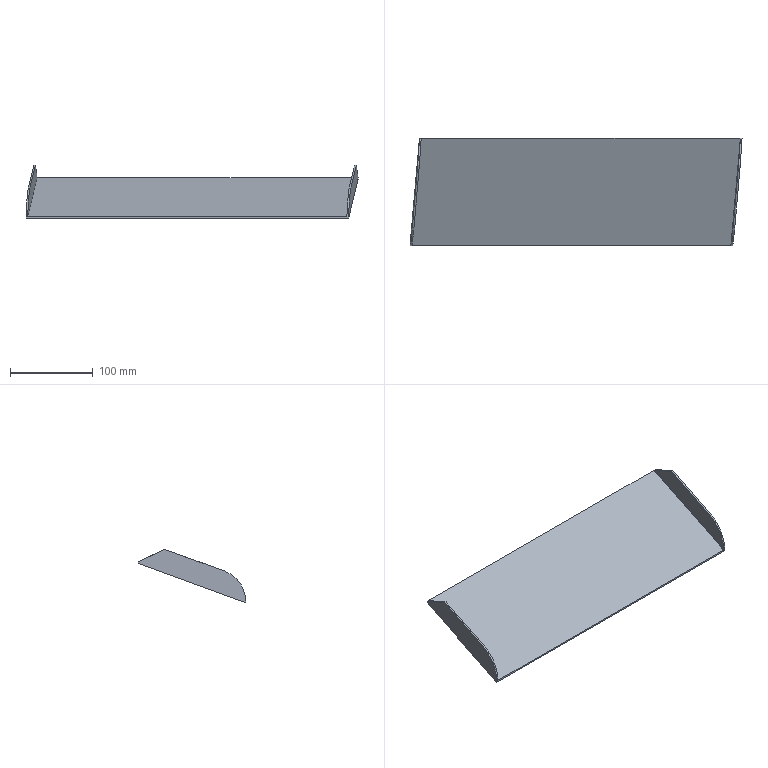Part | NX | features solid 2 | 1 solid | 16 faces | box 400.371 x 130.154 x 64.471 mm | volume 119225 mm3 | plane 14 | cylinder 2 | commonest cylinder face diameters 80 x2
STEP:
#1=CARTESIAN_POINT('',(-476.319,-520.,-137.863));
#2=VERTEX_POINT('',#1);
#3=CARTESIAN_POINT('',(-478.326,-520.,-137.863));
#4=VERTEX_POINT('',#3);
#5=CARTESIAN_POINT('',(-862.915,-520.,-137.863));
#6=DIRECTION('',(1.,0.,0.));
#7=VECTOR('',#6,1000.);
#8=LINE('',#5,#7);
#9=EDGE_CURVE('',#2,#4,#8,.F.);
#10=ORIENTED_EDGE('',*,*,#9,.F.);
#11=CARTESIAN_POINT('',(-476.319,-520.,-139.992));
#12=VERTEX_POINT('',#11);
#13=CARTESIAN_POINT('',(-476.319,-520.,-105.));
#14=DIRECTION('',(0.,0.,1.));
#15=VECTOR('',#14,1000.);
#16=LINE('',#13,#15);
#17=EDGE_CURVE('',#2,#12,#16,.F.);
#18=ORIENTED_EDGE('',*,*,#17,.T.);
#19=CARTESIAN_POINT('',(-865.317,-520.,-139.992));
#20=VERTEX_POINT('',#19);
#21=CARTESIAN_POINT('',(-862.915,-520.,-139.992));
#22=DIRECTION('',(1.,0.,0.));
#23=VECTOR('',#22,1000.);
#24=LINE('',#21,#23);
#25=EDGE_CURVE('',#20,#12,#24,.T.);
#26=ORIENTED_EDGE('',*,*,#25,.F.);
#27=CARTESIAN_POINT('',(-865.257,-520.,-137.863));
#28=VERTEX_POINT('',#27);
#29=CARTESIAN_POINT('',(-865.034,-520.,-129.94));
#30=DIRECTION('',(-0.02811,0.,-0.9996));
#31=VECTOR('',#30,1000.);
#32=LINE('',#29,#31);
#33=EDGE_CURVE('',#28,#20,#32,.T.);
#34=ORIENTED_EDGE('',*,*,#33,.F.);
#35=CARTESIAN_POINT('',(-862.915,-520.,-137.863));
#36=DIRECTION('',(1.,0.,0.));
#37=VECTOR('',#36,1000.);
#38=LINE('',#35,#37);
#39=EDGE_CURVE('',#4,#28,#38,.F.);
#40=ORIENTED_EDGE('',*,*,#39,.F.);
#41=EDGE_LOOP('',(#10,#18,#26,#34,#40));
#42=FACE_BOUND('',#41,.T.);
#43=CARTESIAN_POINT('',(-395.,-520.,0.));
#44=DIRECTION('',(0.,1.,0.));
#45=DIRECTION('',(0.,0.,1.));
#46=AXIS2_PLACEMENT_3D('',#43,#44,#45);
#47=PLANE('',#46);
#48=ADVANCED_FACE('',(#42),#47,.T.);
#49=CARTESIAN_POINT('',(-876.69,-650.,-187.308));
#50=VERTEX_POINT('',#49);
#51=CARTESIAN_POINT('',(-876.63,-650.,-185.179));
#52=VERTEX_POINT('',#51);
#53=CARTESIAN_POINT('',(-875.069,-650.,-129.658));
#54=DIRECTION('',(-0.02811,0.,-0.9996));
#55=VECTOR('',#54,1000.);
#56=LINE('',#53,#55);
#57=EDGE_CURVE('',#50,#52,#56,.F.);
#58=ORIENTED_EDGE('',*,*,#57,.F.);
#59=CARTESIAN_POINT('',(-487.693,-650.,-187.308));
#60=VERTEX_POINT('',#59);
#61=CARTESIAN_POINT('',(50.,-650.,-187.308));
#62=DIRECTION('',(-1.,0.,0.));
#63=VECTOR('',#62,1000.);
#64=LINE('',#61,#63);
#65=EDGE_CURVE('',#50,#60,#64,.F.);
#66=ORIENTED_EDGE('',*,*,#65,.T.);
#67=CARTESIAN_POINT('',(-487.693,-650.,-185.179));
#68=VERTEX_POINT('',#67);
#69=CARTESIAN_POINT('',(-487.693,-650.,-105.));
#70=DIRECTION('',(0.,0.,1.));
#71=VECTOR('',#70,1000.);
#72=LINE('',#69,#71);
#73=EDGE_CURVE('',#60,#68,#72,.T.);
#74=ORIENTED_EDGE('',*,*,#73,.T.);
#75=CARTESIAN_POINT('',(-489.699,-650.,-185.179));
#76=VERTEX_POINT('',#75);
#77=CARTESIAN_POINT('',(-476.319,-650.,-185.179));
#78=DIRECTION('',(1.,0.,0.));
#79=VECTOR('',#78,1000.);
#80=LINE('',#77,#79);
#81=EDGE_CURVE('',#68,#76,#80,.F.);
#82=ORIENTED_EDGE('',*,*,#81,.T.);
#83=CARTESIAN_POINT('',(-874.624,-650.,-185.179));
#84=VERTEX_POINT('',#83);
#85=CARTESIAN_POINT('',(-862.915,-650.,-185.179));
#86=DIRECTION('',(1.,0.,0.));
#87=VECTOR('',#86,1000.);
#88=LINE('',#85,#87);
#89=EDGE_CURVE('',#84,#76,#88,.T.);
#90=ORIENTED_EDGE('',*,*,#89,.F.);
#91=CARTESIAN_POINT('',(-862.915,-650.,-185.179));
#92=DIRECTION('',(1.,0.,0.));
#93=VECTOR('',#92,1000.);
#94=LINE('',#91,#93);
#95=EDGE_CURVE('',#52,#84,#94,.T.);
#96=ORIENTED_EDGE('',*,*,#95,.F.);
#97=EDGE_LOOP('',(#58,#66,#74,#82,#90,#96));
#98=FACE_BOUND('',#97,.T.);
#99=CARTESIAN_POINT('',(50.,-650.,-570.));
#100=DIRECTION('',(0.,1.,0.));
#101=DIRECTION('',(-1.,0.,0.));
#102=AXIS2_PLACEMENT_3D('',#99,#100,#101);
#103=PLANE('',#102);
#104=ADVANCED_FACE('',(#98),#103,.F.);
#105=CARTESIAN_POINT('',(-867.305,-551.964,-122.893));
#106=VERTEX_POINT('',#105);
#107=CARTESIAN_POINT('',(-873.582,-623.706,-149.005));
#108=VERTEX_POINT('',#107);
#109=CARTESIAN_POINT('',(-865.257,-528.551,-114.371));
#110=DIRECTION('',(-0.08194,-0.9365,-0.3409));
#111=VECTOR('',#110,1000.);
#112=LINE('',#109,#111);
#113=EDGE_CURVE('',#106,#108,#112,.T.);
#114=ORIENTED_EDGE('',*,*,#113,.F.);
#115=CARTESIAN_POINT('',(-864.004,-500.45,-147.02));
#116=DIRECTION('',(-0.05794,-0.9041,0.4234));
#117=VECTOR('',#116,1000.);
#118=LINE('',#115,#117);
#119=EDGE_CURVE('',#106,#28,#118,.F.);
#120=ORIENTED_EDGE('',*,*,#119,.T.);
#121=ORIENTED_EDGE('',*,*,#33,.T.);
#122=CARTESIAN_POINT('',(-862.915,-492.548,-130.));
#123=DIRECTION('',(-0.08194,-0.9365,-0.3409));
#124=VECTOR('',#123,1000.);
#125=LINE('',#122,#124);
#126=EDGE_CURVE('',#20,#50,#125,.T.);
#127=ORIENTED_EDGE('',*,*,#126,.T.);
#128=ORIENTED_EDGE('',*,*,#57,.T.);
#129=CARTESIAN_POINT('',(-873.582,-610.025,-186.592));
#130=DIRECTION('',(-0.9966,0.07699,0.02802));
#131=DIRECTION('',(-0.08194,-0.9365,-0.3409));
#132=AXIS2_PLACEMENT_3D('',#129,#130,#131);
#133=ELLIPSE('',#132,40.135,40.);
#134=EDGE_CURVE('',#52,#108,#133,.T.);
#135=ORIENTED_EDGE('',*,*,#134,.T.);
#136=EDGE_LOOP('',(#114,#120,#121,#127,#128,#135));
#137=FACE_BOUND('',#136,.T.);
#138=CARTESIAN_POINT('',(-862.915,-492.548,-130.));
#139=DIRECTION('',(-0.9966,0.07699,0.02802));
#140=DIRECTION('',(-0.07702,-0.997,0.));
#141=AXIS2_PLACEMENT_3D('',#138,#139,#140);
#142=PLANE('',#141);
#143=ADVANCED_FACE('',(#137),#142,.T.);
#144=ORIENTED_EDGE('',*,*,#17,.F.);
#145=CARTESIAN_POINT('',(-476.588,-523.078,-138.983));
#146=DIRECTION('',(-0.08194,-0.9365,-0.3409));
#147=VECTOR('',#146,1000.);
#148=LINE('',#145,#147);
#149=EDGE_CURVE('',#2,#68,#148,.T.);
#150=ORIENTED_EDGE('',*,*,#149,.T.);
#151=ORIENTED_EDGE('',*,*,#73,.F.);
#152=CARTESIAN_POINT('',(-481.762,-582.21,-162.634));
#153=DIRECTION('',(0.08194,0.9365,0.3409));
#154=VECTOR('',#153,1000.);
#155=LINE('',#152,#154);
#156=EDGE_CURVE('',#12,#60,#155,.F.);
#157=ORIENTED_EDGE('',*,*,#156,.F.);
#158=EDGE_LOOP('',(#144,#150,#151,#157));
#159=FACE_BOUND('',#158,.T.);
#160=CARTESIAN_POINT('',(-483.583,-603.028,-105.));
#161=DIRECTION('',(0.9962,-0.08716,0.));
#162=DIRECTION('',(0.08716,0.9962,0.));
#163=AXIS2_PLACEMENT_3D('',#160,#161,#162);
#164=PLANE('',#163);
#165=ADVANCED_FACE('',(#159),#164,.T.);
#166=CARTESIAN_POINT('',(-478.582,-522.924,-138.927));
#167=DIRECTION('',(0.08194,0.9365,0.3409));
#168=VECTOR('',#167,1000.);
#169=LINE('',#166,#168);
#170=EDGE_CURVE('',#4,#76,#169,.F.);
#171=ORIENTED_EDGE('',*,*,#170,.F.);
#172=ORIENTED_EDGE('',*,*,#39,.T.);
#173=CARTESIAN_POINT('',(-863.264,-520.154,-137.919));
#174=VERTEX_POINT('',#173);
#175=CARTESIAN_POINT('',(-865.257,-520.,-137.863));
#176=DIRECTION('',(0.9966,-0.07699,-0.02802));
#177=VECTOR('',#176,1000.);
#178=LINE('',#175,#177);
#179=EDGE_CURVE('',#28,#174,#178,.T.);
#180=ORIENTED_EDGE('',*,*,#179,.T.);
#181=CARTESIAN_POINT('',(-863.264,-520.154,-137.919));
#182=DIRECTION('',(-0.08194,-0.9365,-0.3409));
#183=VECTOR('',#182,1000.);
#184=LINE('',#181,#183);
#185=EDGE_CURVE('',#174,#84,#184,.T.);
#186=ORIENTED_EDGE('',*,*,#185,.T.);
#187=ORIENTED_EDGE('',*,*,#89,.T.);
#188=EDGE_LOOP('',(#171,#172,#180,#186,#187));
#189=FACE_BOUND('',#188,.T.);
#190=CARTESIAN_POINT('',(-862.915,-493.232,-128.121));
#191=DIRECTION('',(0.,0.342,-0.9397));
#192=DIRECTION('',(-0.08194,-0.9365,-0.3409));
#193=AXIS2_PLACEMENT_3D('',#190,#191,#192);
#194=PLANE('',#193);
#195=ADVANCED_FACE('',(#189),#194,.F.);
#196=ORIENTED_EDGE('',*,*,#126,.F.);
#197=ORIENTED_EDGE('',*,*,#25,.T.);
#198=ORIENTED_EDGE('',*,*,#156,.T.);
#199=ORIENTED_EDGE('',*,*,#65,.F.);
#200=EDGE_LOOP('',(#196,#197,#198,#199));
#201=FACE_BOUND('',#200,.T.);
#202=CARTESIAN_POINT('',(-862.915,-492.548,-130.));
#203=DIRECTION('',(0.,0.342,-0.9397));
#204=DIRECTION('',(-0.08194,-0.9365,-0.3409));
#205=AXIS2_PLACEMENT_3D('',#202,#203,#204);
#206=PLANE('',#205);
#207=ADVANCED_FACE('',(#201),#206,.T.);
#208=CARTESIAN_POINT('',(-865.312,-552.118,-122.949));
#209=VERTEX_POINT('',#208);
#210=CARTESIAN_POINT('',(-871.575,-623.706,-149.005));
#211=VERTEX_POINT('',#210);
#212=CARTESIAN_POINT('',(-863.264,-528.704,-114.427));
#213=DIRECTION('',(-0.08194,-0.9365,-0.3409));
#214=VECTOR('',#213,1000.);
#215=LINE('',#212,#214);
#216=EDGE_CURVE('',#209,#211,#215,.T.);
#217=ORIENTED_EDGE('',*,*,#216,.F.);
#218=CARTESIAN_POINT('',(-867.305,-551.964,-122.893));
#219=DIRECTION('',(0.9966,-0.07699,-0.02802));
#220=VECTOR('',#219,1000.);
#221=LINE('',#218,#220);
#222=EDGE_CURVE('',#209,#106,#221,.F.);
#223=ORIENTED_EDGE('',*,*,#222,.T.);
#224=ORIENTED_EDGE('',*,*,#113,.T.);
#225=CARTESIAN_POINT('',(-873.875,-623.706,-149.005));
#226=DIRECTION('',(-1.,0.,0.));
#227=VECTOR('',#226,1000.);
#228=LINE('',#225,#227);
#229=EDGE_CURVE('',#108,#211,#228,.F.);
#230=ORIENTED_EDGE('',*,*,#229,.T.);
#231=EDGE_LOOP('',(#217,#223,#224,#230));
#232=FACE_BOUND('',#231,.T.);
#233=CARTESIAN_POINT('',(-865.257,-528.551,-114.371));
#234=DIRECTION('',(0.,0.342,-0.9397));
#235=DIRECTION('',(-0.08194,-0.9365,-0.3409));
#236=AXIS2_PLACEMENT_3D('',#233,#234,#235);
#237=PLANE('',#236);
#238=ADVANCED_FACE('',(#232),#237,.F.);
#239=ORIENTED_EDGE('',*,*,#185,.F.);
#240=CARTESIAN_POINT('',(-863.264,-520.154,-137.919));
#241=DIRECTION('',(0.05794,0.9041,-0.4234));
#242=VECTOR('',#241,1000.);
#243=LINE('',#240,#242);
#244=EDGE_CURVE('',#174,#209,#243,.F.);
#245=ORIENTED_EDGE('',*,*,#244,.T.);
#246=ORIENTED_EDGE('',*,*,#216,.T.);
#247=CARTESIAN_POINT('',(-871.575,-610.025,-186.592));
#248=DIRECTION('',(-0.9966,0.07699,0.02802));
#249=DIRECTION('',(-0.08194,-0.9365,-0.3409));
#250=AXIS2_PLACEMENT_3D('',#247,#248,#249);
#251=ELLIPSE('',#250,40.135,40.);
#252=EDGE_CURVE('',#211,#84,#251,.F.);
#253=ORIENTED_EDGE('',*,*,#252,.T.);
#254=EDGE_LOOP('',(#239,#245,#246,#253));
#255=FACE_BOUND('',#254,.T.);
#256=CARTESIAN_POINT('',(-863.264,-520.154,-137.919));
#257=DIRECTION('',(-0.9966,0.07699,0.02802));
#258=DIRECTION('',(-0.07702,-0.997,0.));
#259=AXIS2_PLACEMENT_3D('',#256,#257,#258);
#260=PLANE('',#259);
#261=ADVANCED_FACE('',(#255),#260,.F.);
#262=ORIENTED_EDGE('',*,*,#134,.F.);
#263=ORIENTED_EDGE('',*,*,#95,.T.);
#264=ORIENTED_EDGE('',*,*,#252,.F.);
#265=ORIENTED_EDGE('',*,*,#229,.F.);
#266=EDGE_LOOP('',(#262,#263,#264,#265));
#267=FACE_BOUND('',#266,.T.);
#268=CARTESIAN_POINT('',(50.,-610.025,-186.592));
#269=DIRECTION('',(-1.,0.,0.));
#270=DIRECTION('',(0.,0.,1.));
#271=AXIS2_PLACEMENT_3D('',#268,#269,#270);
#272=CYLINDRICAL_SURFACE('',#271,40.);
#273=ADVANCED_FACE('',(#267),#272,.T.);
#274=ORIENTED_EDGE('',*,*,#9,.T.);
#275=CARTESIAN_POINT('',(-478.312,-519.846,-137.807));
#276=VERTEX_POINT('',#275);
#277=CARTESIAN_POINT('',(-478.312,-519.846,-137.807));
#278=DIRECTION('',(-0.08194,-0.9365,-0.3409));
#279=VECTOR('',#278,1000.);
#280=LINE('',#277,#279);
#281=EDGE_CURVE('',#276,#4,#280,.T.);
#282=ORIENTED_EDGE('',*,*,#281,.F.);
#283=CARTESIAN_POINT('',(-476.319,-520.,-137.863));
#284=DIRECTION('',(0.9966,-0.07699,-0.02802));
#285=VECTOR('',#284,1000.);
#286=LINE('',#283,#285);
#287=EDGE_CURVE('',#2,#276,#286,.F.);
#288=ORIENTED_EDGE('',*,*,#287,.F.);
#289=EDGE_LOOP('',(#274,#282,#288));
#290=FACE_BOUND('',#289,.T.);
#291=CARTESIAN_POINT('',(-476.319,-520.,-137.863));
#292=DIRECTION('',(0.,0.342,-0.9397));
#293=DIRECTION('',(-0.08194,-0.9365,-0.3409));
#294=AXIS2_PLACEMENT_3D('',#291,#292,#293);
#295=PLANE('',#294);
#296=ADVANCED_FACE('',(#290),#295,.T.);
#297=CARTESIAN_POINT('',(-478.368,-551.964,-122.893));
#298=VERTEX_POINT('',#297);
#299=CARTESIAN_POINT('',(-484.644,-623.706,-149.005));
#300=VERTEX_POINT('',#299);
#301=CARTESIAN_POINT('',(-476.319,-528.551,-114.371));
#302=DIRECTION('',(-0.08194,-0.9365,-0.3409));
#303=VECTOR('',#302,1000.);
#304=LINE('',#301,#303);
#305=EDGE_CURVE('',#298,#300,#304,.T.);
#306=ORIENTED_EDGE('',*,*,#305,.F.);
#307=CARTESIAN_POINT('',(-480.361,-551.81,-122.837));
#308=VERTEX_POINT('',#307);
#309=CARTESIAN_POINT('',(-478.368,-551.964,-122.893));
#310=DIRECTION('',(-0.9966,0.07699,0.02802));
#311=VECTOR('',#310,1000.);
#312=LINE('',#309,#311);
#313=EDGE_CURVE('',#298,#308,#312,.T.);
#314=ORIENTED_EDGE('',*,*,#313,.T.);
#315=CARTESIAN_POINT('',(-486.651,-623.706,-149.005));
#316=VERTEX_POINT('',#315);
#317=CARTESIAN_POINT('',(-478.312,-528.397,-114.315));
#318=DIRECTION('',(-0.08194,-0.9365,-0.3409));
#319=VECTOR('',#318,1000.);
#320=LINE('',#317,#319);
#321=EDGE_CURVE('',#308,#316,#320,.T.);
#322=ORIENTED_EDGE('',*,*,#321,.T.);
#323=CARTESIAN_POINT('',(-476.319,-623.706,-149.005));
#324=DIRECTION('',(-1.,0.,0.));
#325=VECTOR('',#324,1000.);
#326=LINE('',#323,#325);
#327=EDGE_CURVE('',#316,#300,#326,.F.);
#328=ORIENTED_EDGE('',*,*,#327,.T.);
#329=EDGE_LOOP('',(#306,#314,#322,#328));
#330=FACE_BOUND('',#329,.T.);
#331=CARTESIAN_POINT('',(-476.319,-528.551,-114.371));
#332=DIRECTION('',(0.,0.342,-0.9397));
#333=DIRECTION('',(-0.08194,-0.9365,-0.3409));
#334=AXIS2_PLACEMENT_3D('',#331,#332,#333);
#335=PLANE('',#334);
#336=ADVANCED_FACE('',(#330),#335,.F.);
#337=ORIENTED_EDGE('',*,*,#321,.F.);
#338=CARTESIAN_POINT('',(-478.312,-519.846,-137.807));
#339=DIRECTION('',(-0.05794,-0.9041,0.4234));
#340=VECTOR('',#339,1000.);
#341=LINE('',#338,#340);
#342=EDGE_CURVE('',#308,#276,#341,.F.);
#343=ORIENTED_EDGE('',*,*,#342,.T.);
#344=ORIENTED_EDGE('',*,*,#281,.T.);
#345=ORIENTED_EDGE('',*,*,#170,.T.);
#346=CARTESIAN_POINT('',(-486.651,-610.025,-186.592));
#347=DIRECTION('',(-0.9966,0.07699,0.02802));
#348=DIRECTION('',(-0.08194,-0.9365,-0.3409));
#349=AXIS2_PLACEMENT_3D('',#346,#347,#348);
#350=ELLIPSE('',#349,40.135,40.);
#351=EDGE_CURVE('',#76,#316,#350,.T.);
#352=ORIENTED_EDGE('',*,*,#351,.T.);
#353=EDGE_LOOP('',(#337,#343,#344,#345,#352));
#354=FACE_BOUND('',#353,.T.);
#355=CARTESIAN_POINT('',(-478.312,-519.846,-137.807));
#356=DIRECTION('',(-0.9966,0.07699,0.02802));
#357=DIRECTION('',(-0.07702,-0.997,0.));
#358=AXIS2_PLACEMENT_3D('',#355,#356,#357);
#359=PLANE('',#358);
#360=ADVANCED_FACE('',(#354),#359,.T.);
#361=ORIENTED_EDGE('',*,*,#149,.F.);
#362=CARTESIAN_POINT('',(-478.368,-551.964,-122.893));
#363=DIRECTION('',(0.05794,0.9041,-0.4234));
#364=VECTOR('',#363,1000.);
#365=LINE('',#362,#364);
#366=EDGE_CURVE('',#2,#298,#365,.F.);
#367=ORIENTED_EDGE('',*,*,#366,.T.);
#368=ORIENTED_EDGE('',*,*,#305,.T.);
#369=CARTESIAN_POINT('',(-484.644,-610.025,-186.592));
#370=DIRECTION('',(-0.9966,0.07699,0.02802));
#371=DIRECTION('',(-0.08194,-0.9365,-0.3409));
#372=AXIS2_PLACEMENT_3D('',#369,#370,#371);
#373=ELLIPSE('',#372,40.135,40.);
#374=EDGE_CURVE('',#300,#68,#373,.F.);
#375=ORIENTED_EDGE('',*,*,#374,.T.);
#376=EDGE_LOOP('',(#361,#367,#368,#375));
#377=FACE_BOUND('',#376,.T.);
#378=CARTESIAN_POINT('',(-476.319,-520.,-137.863));
#379=DIRECTION('',(-0.9966,0.07699,0.02802));
#380=DIRECTION('',(-0.07702,-0.997,0.));
#381=AXIS2_PLACEMENT_3D('',#378,#379,#380);
#382=PLANE('',#381);
#383=ADVANCED_FACE('',(#377),#382,.F.);
#384=ORIENTED_EDGE('',*,*,#374,.F.);
#385=ORIENTED_EDGE('',*,*,#327,.F.);
#386=ORIENTED_EDGE('',*,*,#351,.F.);
#387=ORIENTED_EDGE('',*,*,#81,.F.);
#388=EDGE_LOOP('',(#384,#385,#386,#387));
#389=FACE_BOUND('',#388,.T.);
#390=CARTESIAN_POINT('',(50.,-610.025,-186.592));
#391=DIRECTION('',(-1.,0.,0.));
#392=DIRECTION('',(0.,0.,1.));
#393=AXIS2_PLACEMENT_3D('',#390,#391,#392);
#394=CYLINDRICAL_SURFACE('',#393,40.);
#395=ADVANCED_FACE('',(#389),#394,.T.);
#396=ORIENTED_EDGE('',*,*,#119,.F.);
#397=ORIENTED_EDGE('',*,*,#222,.F.);
#398=ORIENTED_EDGE('',*,*,#244,.F.);
#399=ORIENTED_EDGE('',*,*,#179,.F.);
#400=EDGE_LOOP('',(#396,#397,#398,#399));
#401=FACE_BOUND('',#400,.T.);
#402=CARTESIAN_POINT('',(-865.257,-520.,-137.863));
#403=DIRECTION('',(-0.05794,-0.4204,-0.9055));
#404=DIRECTION('',(0.,0.907,-0.4211));
#405=AXIS2_PLACEMENT_3D('',#402,#403,#404);
#406=PLANE('',#405);
#407=ADVANCED_FACE('',(#401),#406,.F.);
#408=ORIENTED_EDGE('',*,*,#366,.F.);
#409=ORIENTED_EDGE('',*,*,#287,.T.);
#410=ORIENTED_EDGE('',*,*,#342,.F.);
#411=ORIENTED_EDGE('',*,*,#313,.F.);
#412=EDGE_LOOP('',(#408,#409,#410,#411));
#413=FACE_BOUND('',#412,.T.);
#414=CARTESIAN_POINT('',(-478.368,-551.964,-122.893));
#415=DIRECTION('',(-0.05794,-0.4204,-0.9055));
#416=DIRECTION('',(0.,0.907,-0.4211));
#417=AXIS2_PLACEMENT_3D('',#414,#415,#416);
#418=PLANE('',#417);
#419=ADVANCED_FACE('',(#413),#418,.F.);
#420=CLOSED_SHELL('',(#48,#104,#143,#165,#195,#207,#238,#261,#273,#296,#336,#360,#383,#395,#407,#419));
#421=MANIFOLD_SOLID_BREP('',#420);
#422=(LENGTH_UNIT()NAMED_UNIT(*)SI_UNIT(.MILLI.,.METRE.));
#423=UNCERTAINTY_MEASURE_WITH_UNIT(LENGTH_MEASURE(0.00001),#422,'','');
#424=(NAMED_UNIT(*)PLANE_ANGLE_UNIT()SI_UNIT($,.RADIAN.));
#425=(NAMED_UNIT(*)SI_UNIT($,.STERADIAN.)SOLID_ANGLE_UNIT());
#426=(GEOMETRIC_REPRESENTATION_CONTEXT(3)GLOBAL_UNCERTAINTY_ASSIGNED_CONTEXT((#423))GLOBAL_UNIT_ASSIGNED_CONTEXT((#422,#424,#425))REPRESENTATION_CONTEXT('',''));
#427=ADVANCED_BREP_SHAPE_REPRESENTATION('',(#421),#426);